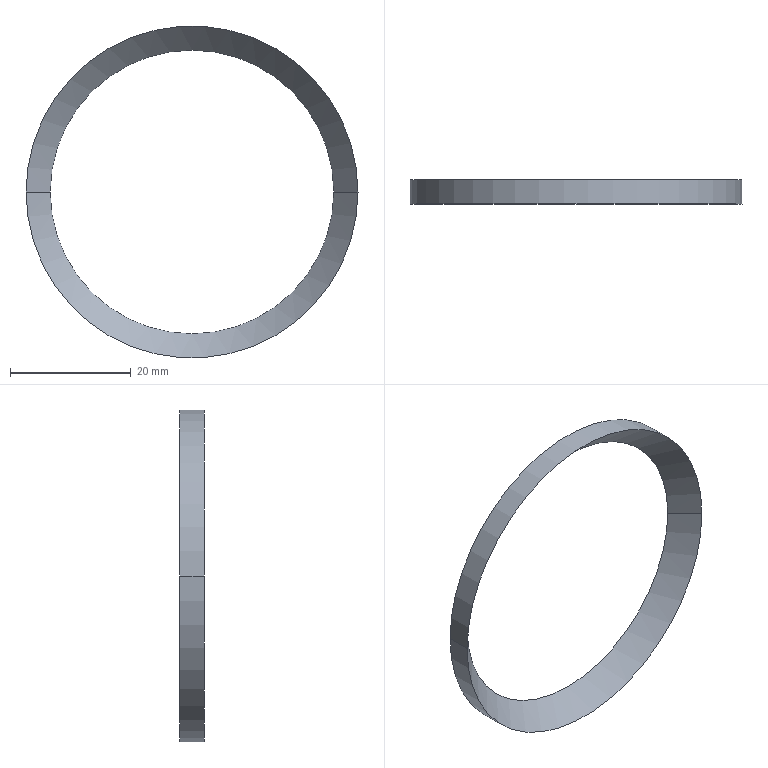Part | SolidWorks | 1 solid | 5 faces | box 55 x 4 x 55 mm | volume 1315 mm3 | cylinder 2 | cone 2 | plane 1 | commonest cylinder face diameters 55 x2
STEP:
#1=CARTESIAN_POINT('',(-22.701,48.795,0.));
#2=VERTEX_POINT('',#1);
#3=CARTESIAN_POINT('',(32.299,48.795,0.));
#4=VERTEX_POINT('',#3);
#5=CARTESIAN_POINT('',(4.799,48.795,0.));
#6=DIRECTION('',(0.,-1.,0.));
#7=DIRECTION('',(-1.,0.,0.));
#8=AXIS2_PLACEMENT_3D('',#5,#6,#7);
#9=CIRCLE('',#8,27.5);
#10=EDGE_CURVE('',#2,#4,#9,.T.);
#11=ORIENTED_EDGE('',*,*,#10,.T.);
#12=CARTESIAN_POINT('',(32.299,44.795,0.));
#13=VERTEX_POINT('',#12);
#14=CARTESIAN_POINT('',(32.299,48.795,0.));
#15=DIRECTION('',(0.,-1.,0.));
#16=VECTOR('',#15,1000.);
#17=LINE('',#14,#16);
#18=EDGE_CURVE('',#4,#13,#17,.T.);
#19=ORIENTED_EDGE('',*,*,#18,.T.);
#20=CARTESIAN_POINT('',(-22.701,44.795,0.));
#21=VERTEX_POINT('',#20);
#22=CARTESIAN_POINT('',(4.799,44.795,0.));
#23=DIRECTION('',(0.,1.,0.));
#24=DIRECTION('',(1.,0.,0.));
#25=AXIS2_PLACEMENT_3D('',#22,#23,#24);
#26=CIRCLE('',#25,27.5);
#27=EDGE_CURVE('',#13,#21,#26,.T.);
#28=ORIENTED_EDGE('',*,*,#27,.T.);
#29=CARTESIAN_POINT('',(-22.701,48.795,0.));
#30=DIRECTION('',(0.,-1.,0.));
#31=VECTOR('',#30,1000.);
#32=LINE('',#29,#31);
#33=EDGE_CURVE('',#2,#21,#32,.T.);
#34=ORIENTED_EDGE('',*,*,#33,.F.);
#35=EDGE_LOOP('',(#11,#19,#28,#34));
#36=FACE_OUTER_BOUND('',#35,.T.);
#37=CARTESIAN_POINT('',(4.799,40.795,0.));
#38=DIRECTION('',(0.,1.,0.));
#39=DIRECTION('',(1.,0.,0.));
#40=AXIS2_PLACEMENT_3D('',#37,#38,#39);
#41=CYLINDRICAL_SURFACE('',#40,27.5);
#42=ADVANCED_FACE('',(#36),#41,.T.);
#43=CARTESIAN_POINT('',(-18.701,48.795,0.));
#44=VERTEX_POINT('',#43);
#45=CARTESIAN_POINT('',(-22.701,44.795,0.));
#46=DIRECTION('',(0.7071,0.7071,0.));
#47=VECTOR('',#46,1000.);
#48=LINE('',#45,#47);
#49=EDGE_CURVE('',#21,#44,#48,.T.);
#50=ORIENTED_EDGE('',*,*,#49,.F.);
#51=ORIENTED_EDGE('',*,*,#27,.F.);
#52=CARTESIAN_POINT('',(28.299,48.795,0.));
#53=VERTEX_POINT('',#52);
#54=CARTESIAN_POINT('',(32.299,44.795,0.));
#55=DIRECTION('',(-0.7071,0.7071,0.));
#56=VECTOR('',#55,1000.);
#57=LINE('',#54,#56);
#58=EDGE_CURVE('',#13,#53,#57,.T.);
#59=ORIENTED_EDGE('',*,*,#58,.T.);
#60=CARTESIAN_POINT('',(4.799,48.795,0.));
#61=DIRECTION('',(0.,1.,0.));
#62=DIRECTION('',(1.,0.,0.));
#63=AXIS2_PLACEMENT_3D('',#60,#61,#62);
#64=CIRCLE('',#63,23.5);
#65=EDGE_CURVE('',#53,#44,#64,.T.);
#66=ORIENTED_EDGE('',*,*,#65,.T.);
#67=EDGE_LOOP('',(#50,#51,#59,#66));
#68=FACE_OUTER_BOUND('',#67,.T.);
#69=CARTESIAN_POINT('',(4.799,48.875,0.));
#70=DIRECTION('',(0.,-1.,0.));
#71=DIRECTION('',(-1.,0.,0.));
#72=AXIS2_PLACEMENT_3D('',#69,#70,#71);
#73=CONICAL_SURFACE('',#72,23.42,0.7854);
#74=ADVANCED_FACE('',(#68),#73,.F.);
#75=CARTESIAN_POINT('',(4.799,44.795,0.));
#76=DIRECTION('',(0.,1.,0.));
#77=DIRECTION('',(-1.,0.,0.));
#78=AXIS2_PLACEMENT_3D('',#75,#76,#77);
#79=CIRCLE('',#78,27.5);
#80=EDGE_CURVE('',#21,#13,#79,.T.);
#81=ORIENTED_EDGE('',*,*,#80,.F.);
#82=ORIENTED_EDGE('',*,*,#49,.T.);
#83=CARTESIAN_POINT('',(4.799,48.795,0.));
#84=DIRECTION('',(0.,1.,0.));
#85=DIRECTION('',(-1.,0.,0.));
#86=AXIS2_PLACEMENT_3D('',#83,#84,#85);
#87=CIRCLE('',#86,23.5);
#88=EDGE_CURVE('',#44,#53,#87,.T.);
#89=ORIENTED_EDGE('',*,*,#88,.T.);
#90=ORIENTED_EDGE('',*,*,#58,.F.);
#91=EDGE_LOOP('',(#81,#82,#89,#90));
#92=FACE_OUTER_BOUND('',#91,.T.);
#93=CARTESIAN_POINT('',(4.799,48.875,0.));
#94=DIRECTION('',(0.,-1.,0.));
#95=DIRECTION('',(-1.,0.,0.));
#96=AXIS2_PLACEMENT_3D('',#93,#94,#95);
#97=CONICAL_SURFACE('',#96,23.42,0.7854);
#98=ADVANCED_FACE('',(#92),#97,.F.);
#99=ORIENTED_EDGE('',*,*,#18,.F.);
#100=CARTESIAN_POINT('',(4.799,48.795,0.));
#101=DIRECTION('',(0.,-1.,0.));
#102=DIRECTION('',(1.,0.,0.));
#103=AXIS2_PLACEMENT_3D('',#100,#101,#102);
#104=CIRCLE('',#103,27.5);
#105=EDGE_CURVE('',#4,#2,#104,.T.);
#106=ORIENTED_EDGE('',*,*,#105,.T.);
#107=ORIENTED_EDGE('',*,*,#33,.T.);
#108=ORIENTED_EDGE('',*,*,#80,.T.);
#109=EDGE_LOOP('',(#99,#106,#107,#108));
#110=FACE_OUTER_BOUND('',#109,.T.);
#111=CARTESIAN_POINT('',(4.799,40.795,0.));
#112=DIRECTION('',(0.,1.,0.));
#113=DIRECTION('',(1.,0.,0.));
#114=AXIS2_PLACEMENT_3D('',#111,#112,#113);
#115=CYLINDRICAL_SURFACE('',#114,27.5);
#116=ADVANCED_FACE('',(#110),#115,.T.);
#117=ORIENTED_EDGE('',*,*,#65,.F.);
#118=ORIENTED_EDGE('',*,*,#88,.F.);
#119=EDGE_LOOP('',(#117,#118));
#120=FACE_BOUND('',#119,.T.);
#121=ORIENTED_EDGE('',*,*,#10,.F.);
#122=ORIENTED_EDGE('',*,*,#105,.F.);
#123=EDGE_LOOP('',(#121,#122));
#124=FACE_OUTER_BOUND('',#123,.T.);
#125=CARTESIAN_POINT('',(-22.701,48.795,0.));
#126=DIRECTION('',(0.,-1.,0.));
#127=DIRECTION('',(0.,0.,-1.));
#128=AXIS2_PLACEMENT_3D('',#125,#126,#127);
#129=PLANE('',#128);
#130=ADVANCED_FACE('',(#120,#124),#129,.F.);
#131=CLOSED_SHELL('',(#42,#74,#98,#116,#130));
#132=MANIFOLD_SOLID_BREP('',#131);
#133=CARTESIAN_POINT('',(0.,0.,0.));
#134=DIRECTION('',(0.,0.,1.));
#135=DIRECTION('',(1.,0.,0.));
#136=AXIS2_PLACEMENT_3D('',#133,#134,#135);
#137=(LENGTH_UNIT()NAMED_UNIT(*)SI_UNIT(.MILLI.,.METRE.));
#138=UNCERTAINTY_MEASURE_WITH_UNIT(LENGTH_MEASURE(0.00001),#137,'','');
#139=(NAMED_UNIT(*)PLANE_ANGLE_UNIT()SI_UNIT($,.RADIAN.));
#140=(NAMED_UNIT(*)SI_UNIT($,.STERADIAN.)SOLID_ANGLE_UNIT());
#141=(GEOMETRIC_REPRESENTATION_CONTEXT(3)GLOBAL_UNCERTAINTY_ASSIGNED_CONTEXT((#138))GLOBAL_UNIT_ASSIGNED_CONTEXT((#137,#139,#140))REPRESENTATION_CONTEXT('',''));
#142=ADVANCED_BREP_SHAPE_REPRESENTATION('',(#132,#136),#141);